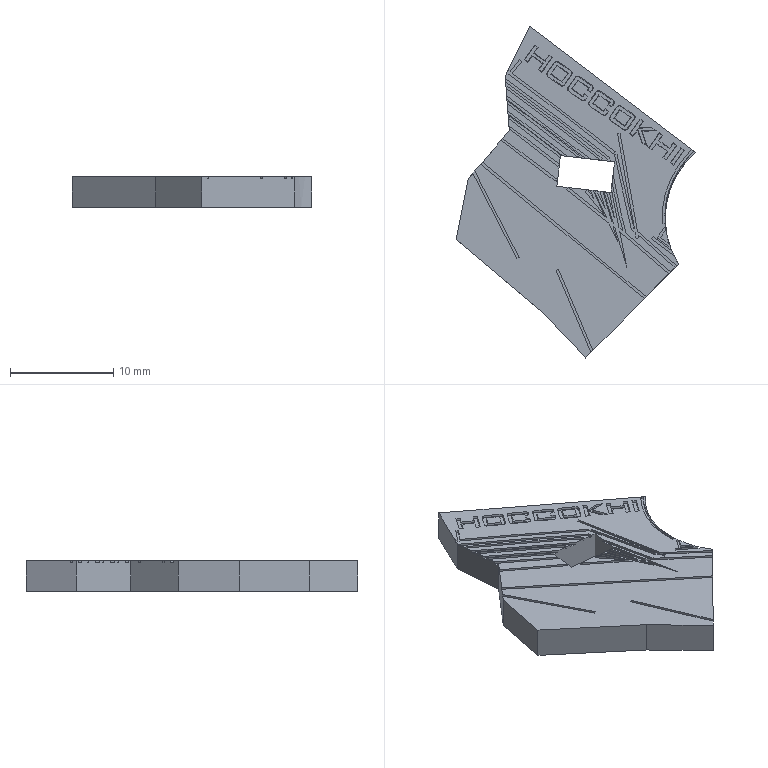Part | SolidWorks | features BaseBody 1 | 1 solid | 264 faces | box 23.207 x 32.146 x 3 mm | volume 1195 mm3 | plane 212 | spline 50 | cylinder 2 | commonest cylinder face diameters 16.634 x2